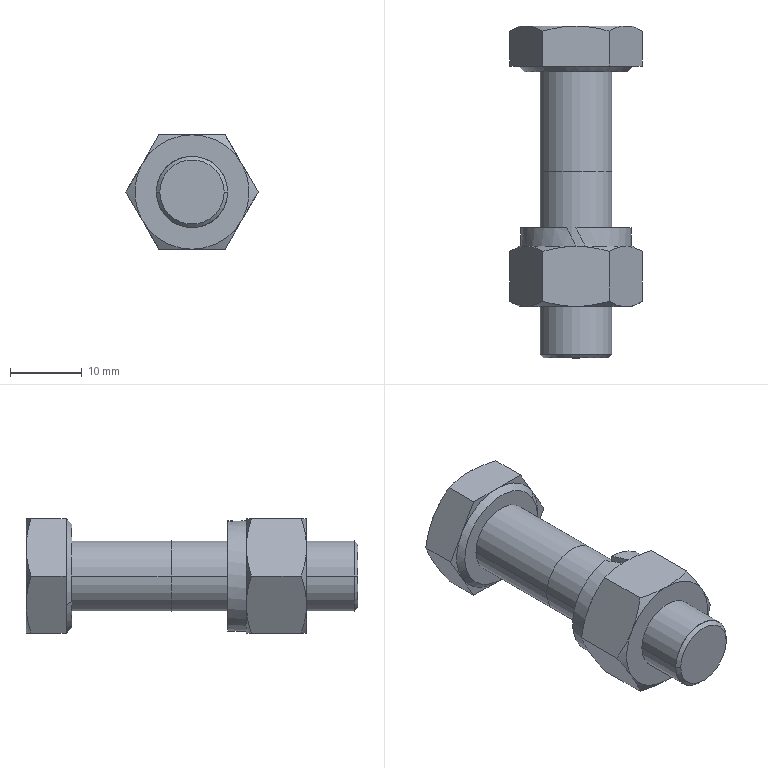Part | NX | features BREP 5 | 3 solids | 67 faces | box 18.475 x 46.4 x 16 mm | volume 7344 mm3 | plane 29 | cone 26 | cylinder 12 | commonest cylinder face diameters 8.376 x4 10 x4 10.2 x2 15.4 x2